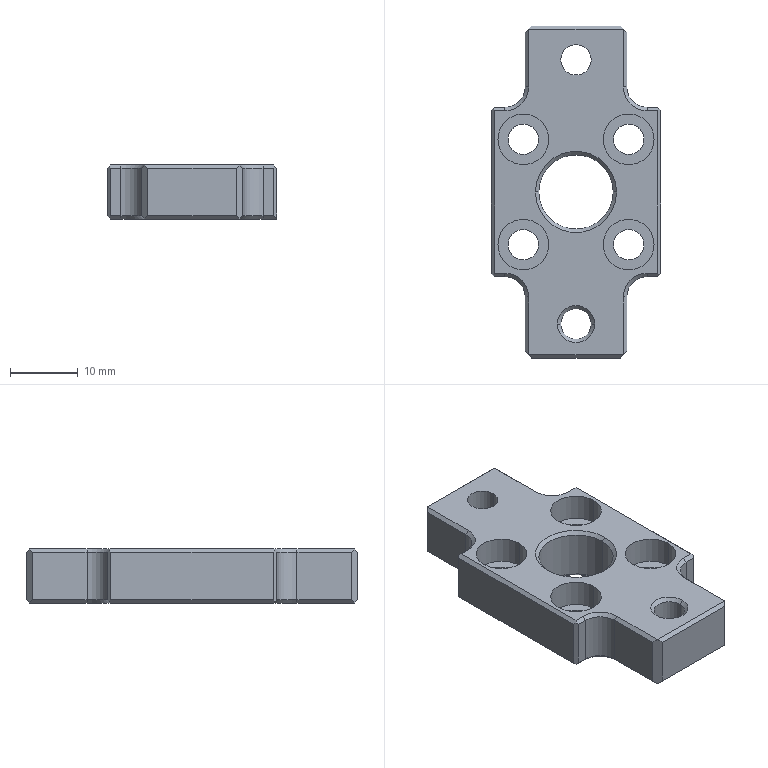Part | SolidWorks | features Chamfer 3, HoleWzd 3, Cut 1, Extrusion 1, Fillet 1, ICE 1 | 1 solid | 95 faces | box 25 x 49 x 8 mm | volume 5678 mm3 | plane 51 | cylinder 30 | cone 14 | commonest cylinder face diameters 4.5 x12 7.5 x12 6 x4 11 x2